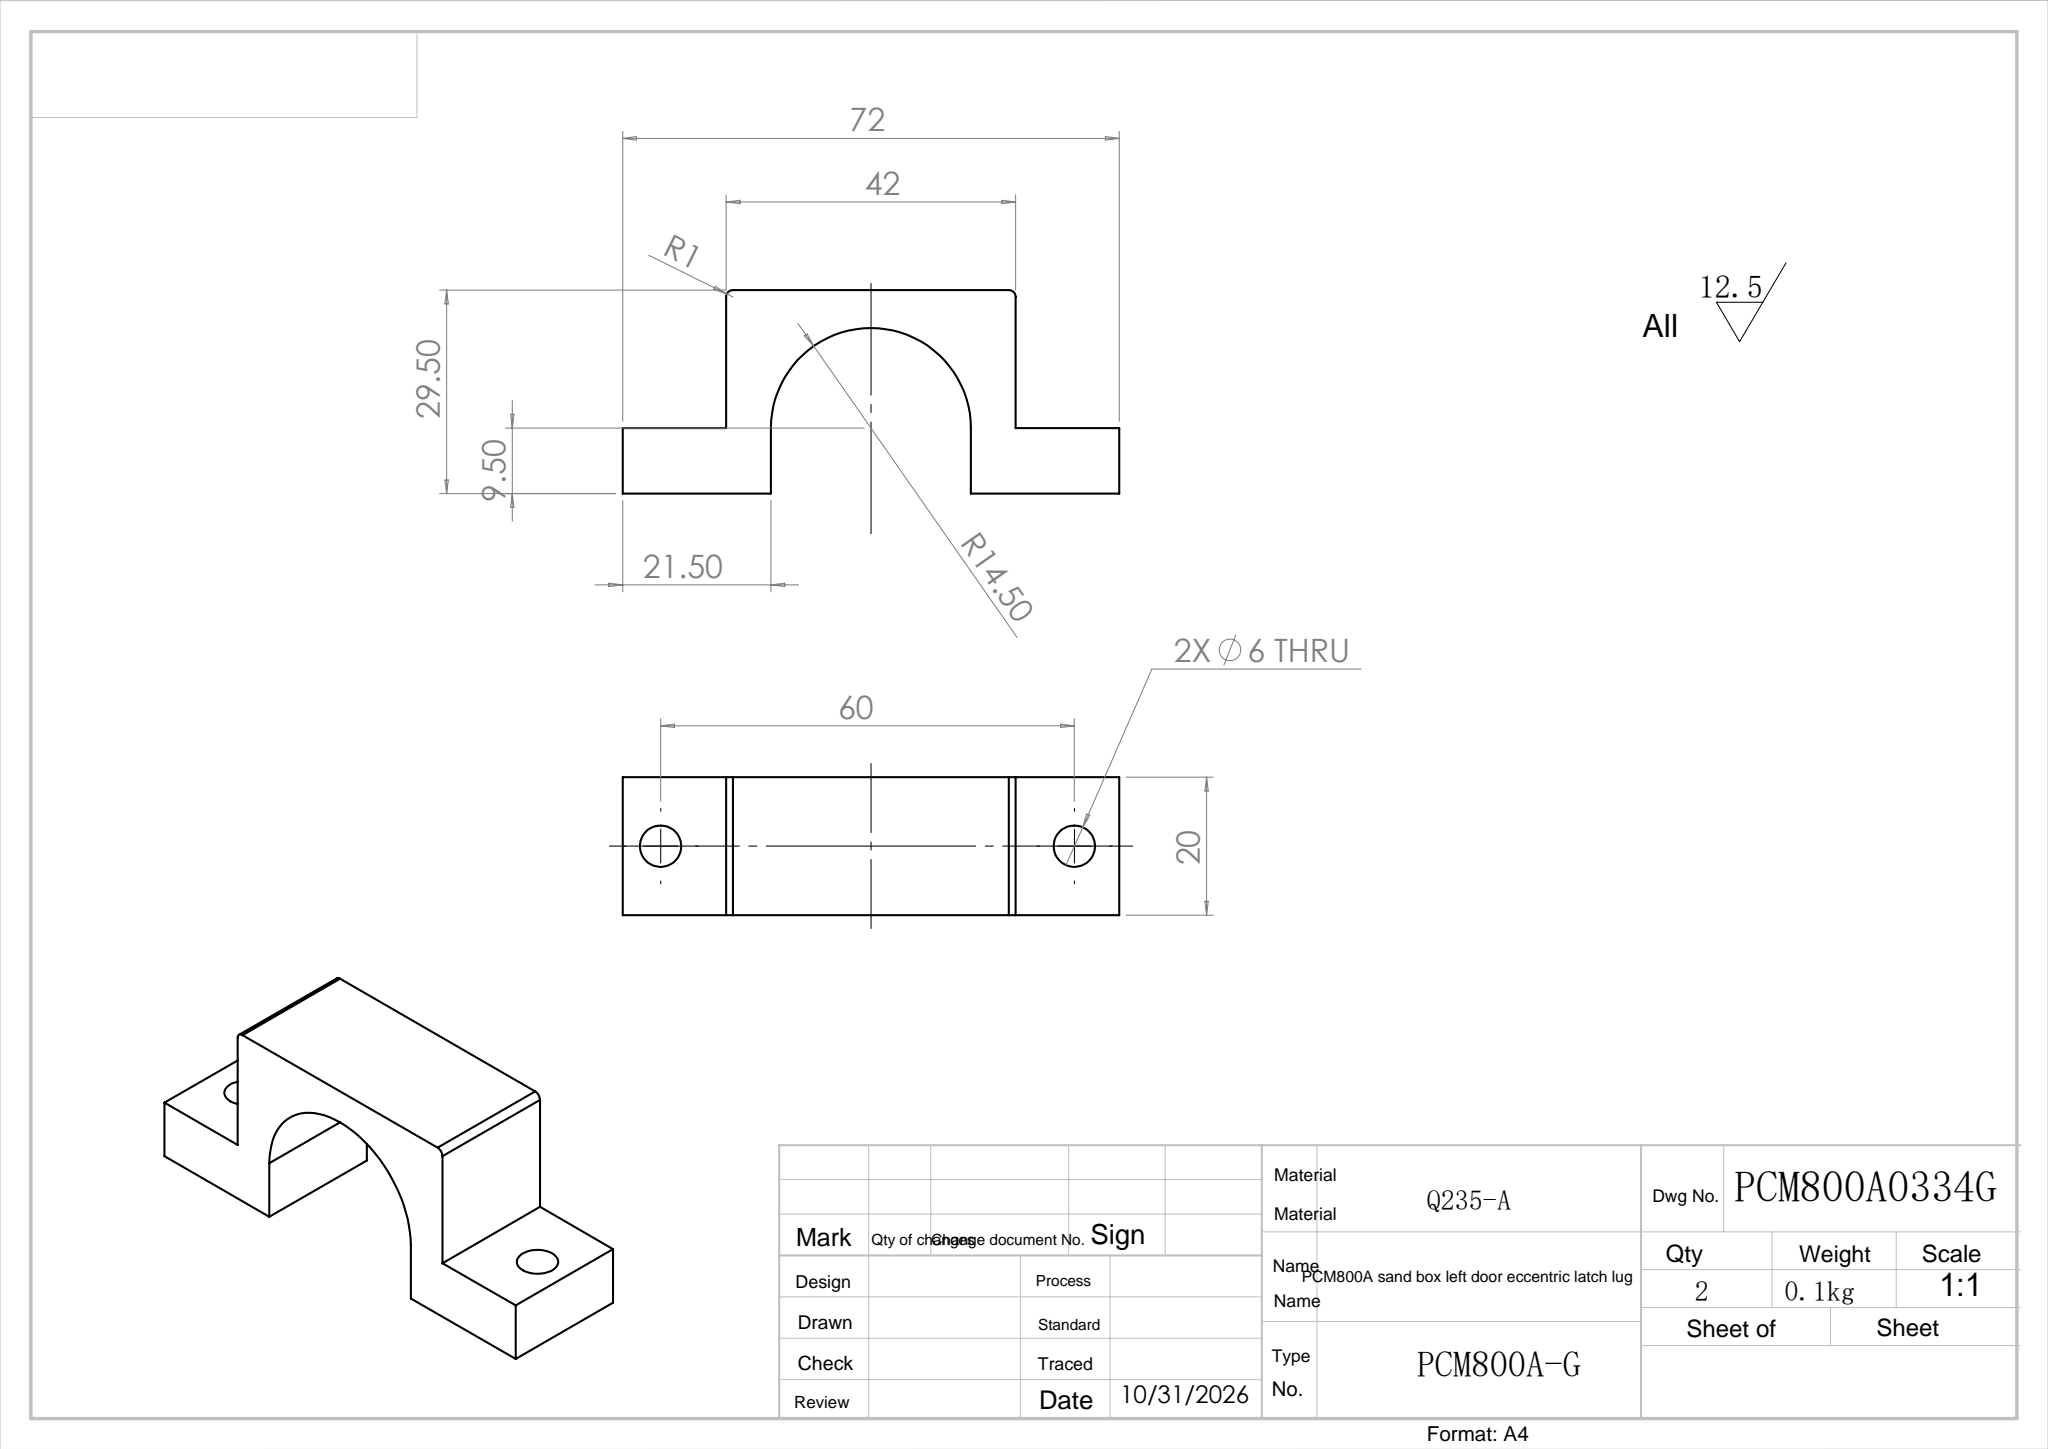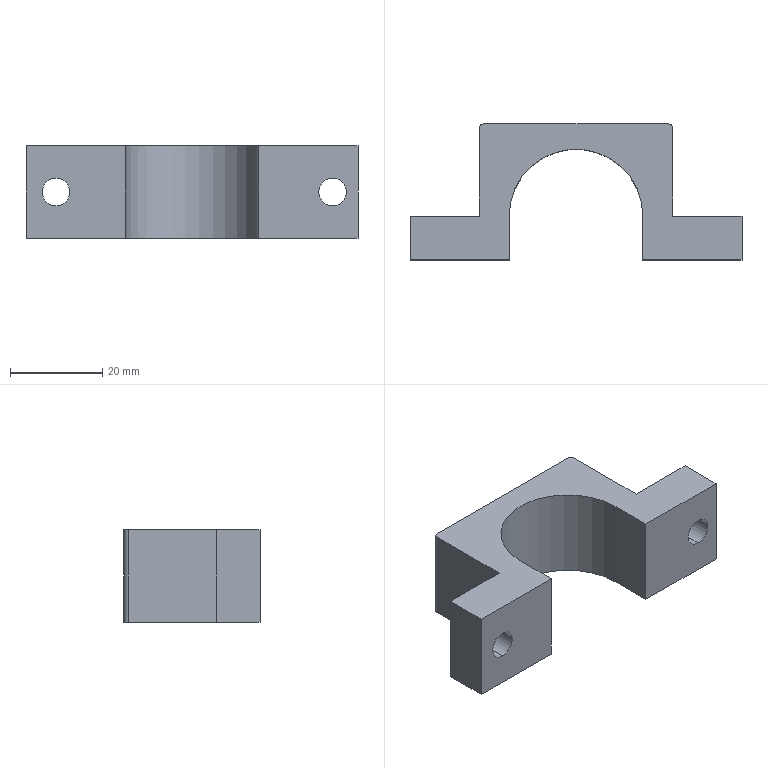Part | SolidWorks | features Extrusion 1, Fillet 1, ICE 1 | 1 solid | 20 faces | box 72 x 29.5 x 20 mm | volume 17819 mm3 | plane 13 | cylinder 7 | commonest cylinder face diameters 6 x4 2 x2 29 x1
STEP:
#1=CARTESIAN_POINT('',(66.5,-9.5,7.));
#2=VERTEX_POINT('',#1);
#3=CARTESIAN_POINT('',(66.5,-9.5,13.));
#4=VERTEX_POINT('',#3);
#5=CARTESIAN_POINT('',(66.5,-9.5,10.));
#6=DIRECTION('',(0.,1.,0.));
#7=DIRECTION('',(0.,0.,1.));
#8=AXIS2_PLACEMENT_3D('',#5,#6,#7);
#9=CIRCLE('',#8,3.);
#10=EDGE_CURVE('',#2,#4,#9,.T.);
#11=ORIENTED_EDGE('',*,*,#10,.F.);
#12=CARTESIAN_POINT('',(66.5,0.,7.));
#13=VERTEX_POINT('',#12);
#14=CARTESIAN_POINT('',(66.5,-9.5,7.));
#15=DIRECTION('',(0.,1.,0.));
#16=VECTOR('',#15,1000.);
#17=LINE('',#14,#16);
#18=EDGE_CURVE('',#2,#13,#17,.T.);
#19=ORIENTED_EDGE('',*,*,#18,.T.);
#20=CARTESIAN_POINT('',(66.5,0.,13.));
#21=VERTEX_POINT('',#20);
#22=CARTESIAN_POINT('',(66.5,0.,10.));
#23=DIRECTION('',(0.,1.,0.));
#24=DIRECTION('',(0.,0.,1.));
#25=AXIS2_PLACEMENT_3D('',#22,#23,#24);
#26=CIRCLE('',#25,3.);
#27=EDGE_CURVE('',#13,#21,#26,.T.);
#28=ORIENTED_EDGE('',*,*,#27,.T.);
#29=CARTESIAN_POINT('',(66.5,-9.5,13.));
#30=DIRECTION('',(0.,1.,0.));
#31=VECTOR('',#30,1000.);
#32=LINE('',#29,#31);
#33=EDGE_CURVE('',#4,#21,#32,.T.);
#34=ORIENTED_EDGE('',*,*,#33,.F.);
#35=EDGE_LOOP('',(#11,#19,#28,#34));
#36=FACE_OUTER_BOUND('',#35,.T.);
#37=CARTESIAN_POINT('',(66.5,-9.5,10.));
#38=DIRECTION('',(0.,1.,0.));
#39=DIRECTION('',(0.,0.,1.));
#40=AXIS2_PLACEMENT_3D('',#37,#38,#39);
#41=CYLINDRICAL_SURFACE('',#40,3.);
#42=ADVANCED_FACE('',(#36),#41,.F.);
#43=CARTESIAN_POINT('',(6.5,-9.5,7.));
#44=VERTEX_POINT('',#43);
#45=CARTESIAN_POINT('',(6.5,-9.5,13.));
#46=VERTEX_POINT('',#45);
#47=CARTESIAN_POINT('',(6.5,-9.5,10.));
#48=DIRECTION('',(0.,1.,0.));
#49=DIRECTION('',(0.,0.,1.));
#50=AXIS2_PLACEMENT_3D('',#47,#48,#49);
#51=CIRCLE('',#50,3.);
#52=EDGE_CURVE('',#44,#46,#51,.T.);
#53=ORIENTED_EDGE('',*,*,#52,.F.);
#54=CARTESIAN_POINT('',(6.5,0.,7.));
#55=VERTEX_POINT('',#54);
#56=CARTESIAN_POINT('',(6.5,-9.5,7.));
#57=DIRECTION('',(0.,1.,0.));
#58=VECTOR('',#57,1000.);
#59=LINE('',#56,#58);
#60=EDGE_CURVE('',#44,#55,#59,.T.);
#61=ORIENTED_EDGE('',*,*,#60,.T.);
#62=CARTESIAN_POINT('',(6.5,0.,13.));
#63=VERTEX_POINT('',#62);
#64=CARTESIAN_POINT('',(6.5,0.,10.));
#65=DIRECTION('',(0.,1.,0.));
#66=DIRECTION('',(0.,0.,1.));
#67=AXIS2_PLACEMENT_3D('',#64,#65,#66);
#68=CIRCLE('',#67,3.);
#69=EDGE_CURVE('',#55,#63,#68,.T.);
#70=ORIENTED_EDGE('',*,*,#69,.T.);
#71=CARTESIAN_POINT('',(6.5,-9.5,13.));
#72=DIRECTION('',(0.,1.,0.));
#73=VECTOR('',#72,1000.);
#74=LINE('',#71,#73);
#75=EDGE_CURVE('',#46,#63,#74,.T.);
#76=ORIENTED_EDGE('',*,*,#75,.F.);
#77=EDGE_LOOP('',(#53,#61,#70,#76));
#78=FACE_OUTER_BOUND('',#77,.T.);
#79=CARTESIAN_POINT('',(6.5,-9.5,10.));
#80=DIRECTION('',(0.,1.,0.));
#81=DIRECTION('',(0.,0.,1.));
#82=AXIS2_PLACEMENT_3D('',#79,#80,#81);
#83=CYLINDRICAL_SURFACE('',#82,3.);
#84=ADVANCED_FACE('',(#78),#83,.F.);
#85=CARTESIAN_POINT('',(0.,0.,0.));
#86=VERTEX_POINT('',#85);
#87=CARTESIAN_POINT('',(0.,-9.5,0.));
#88=VERTEX_POINT('',#87);
#89=CARTESIAN_POINT('',(0.,-9.5,0.));
#90=DIRECTION('',(0.,-1.,0.));
#91=VECTOR('',#90,1000.);
#92=LINE('',#89,#91);
#93=EDGE_CURVE('',#86,#88,#92,.T.);
#94=ORIENTED_EDGE('',*,*,#93,.T.);
#95=CARTESIAN_POINT('',(0.,-9.5,20.));
#96=VERTEX_POINT('',#95);
#97=CARTESIAN_POINT('',(0.,-9.5,20.));
#98=DIRECTION('',(0.,0.,-1.));
#99=VECTOR('',#98,1000.);
#100=LINE('',#97,#99);
#101=EDGE_CURVE('',#96,#88,#100,.T.);
#102=ORIENTED_EDGE('',*,*,#101,.F.);
#103=CARTESIAN_POINT('',(0.,0.,20.));
#104=VERTEX_POINT('',#103);
#105=CARTESIAN_POINT('',(0.,-9.5,20.));
#106=DIRECTION('',(0.,-1.,0.));
#107=VECTOR('',#106,1000.);
#108=LINE('',#105,#107);
#109=EDGE_CURVE('',#104,#96,#108,.T.);
#110=ORIENTED_EDGE('',*,*,#109,.F.);
#111=CARTESIAN_POINT('',(0.,0.,20.));
#112=DIRECTION('',(0.,0.,-1.));
#113=VECTOR('',#112,1000.);
#114=LINE('',#111,#113);
#115=EDGE_CURVE('',#104,#86,#114,.T.);
#116=ORIENTED_EDGE('',*,*,#115,.T.);
#117=EDGE_LOOP('',(#94,#102,#110,#116));
#118=FACE_OUTER_BOUND('',#117,.T.);
#119=CARTESIAN_POINT('',(0.,-9.5,20.));
#120=DIRECTION('',(1.,0.,0.));
#121=DIRECTION('',(0.,0.,-1.));
#122=AXIS2_PLACEMENT_3D('',#119,#120,#121);
#123=PLANE('',#122);
#124=ADVANCED_FACE('',(#118),#123,.F.);
#125=CARTESIAN_POINT('',(6.5,-9.5,10.));
#126=DIRECTION('',(0.,1.,0.));
#127=DIRECTION('',(0.,0.,1.));
#128=AXIS2_PLACEMENT_3D('',#125,#126,#127);
#129=CIRCLE('',#128,3.);
#130=EDGE_CURVE('',#46,#44,#129,.T.);
#131=ORIENTED_EDGE('',*,*,#130,.T.);
#132=ORIENTED_EDGE('',*,*,#52,.T.);
#133=EDGE_LOOP('',(#131,#132));
#134=FACE_BOUND('',#133,.T.);
#135=CARTESIAN_POINT('',(21.5,-9.5,0.));
#136=VERTEX_POINT('',#135);
#137=CARTESIAN_POINT('',(21.5,-9.5,0.));
#138=DIRECTION('',(1.,0.,0.));
#139=VECTOR('',#138,1000.);
#140=LINE('',#137,#139);
#141=EDGE_CURVE('',#88,#136,#140,.T.);
#142=ORIENTED_EDGE('',*,*,#141,.T.);
#143=CARTESIAN_POINT('',(21.5,-9.5,20.));
#144=VERTEX_POINT('',#143);
#145=CARTESIAN_POINT('',(21.5,-9.5,20.));
#146=DIRECTION('',(0.,0.,-1.));
#147=VECTOR('',#146,1000.);
#148=LINE('',#145,#147);
#149=EDGE_CURVE('',#144,#136,#148,.T.);
#150=ORIENTED_EDGE('',*,*,#149,.F.);
#151=CARTESIAN_POINT('',(21.5,-9.5,20.));
#152=DIRECTION('',(1.,0.,0.));
#153=VECTOR('',#152,1000.);
#154=LINE('',#151,#153);
#155=EDGE_CURVE('',#96,#144,#154,.T.);
#156=ORIENTED_EDGE('',*,*,#155,.F.);
#157=ORIENTED_EDGE('',*,*,#101,.T.);
#158=EDGE_LOOP('',(#142,#150,#156,#157));
#159=FACE_OUTER_BOUND('',#158,.T.);
#160=CARTESIAN_POINT('',(21.5,-9.5,20.));
#161=DIRECTION('',(0.,1.,0.));
#162=DIRECTION('',(-1.,0.,0.));
#163=AXIS2_PLACEMENT_3D('',#160,#161,#162);
#164=PLANE('',#163);
#165=ADVANCED_FACE('',(#134,#159),#164,.F.);
#166=CARTESIAN_POINT('',(21.5,0.,0.));
#167=VERTEX_POINT('',#166);
#168=CARTESIAN_POINT('',(21.5,0.,0.));
#169=DIRECTION('',(0.,1.,0.));
#170=VECTOR('',#169,1000.);
#171=LINE('',#168,#170);
#172=EDGE_CURVE('',#136,#167,#171,.T.);
#173=ORIENTED_EDGE('',*,*,#172,.T.);
#174=CARTESIAN_POINT('',(21.5,0.,20.));
#175=VERTEX_POINT('',#174);
#176=CARTESIAN_POINT('',(21.5,0.,20.));
#177=DIRECTION('',(0.,0.,-1.));
#178=VECTOR('',#177,1000.);
#179=LINE('',#176,#178);
#180=EDGE_CURVE('',#175,#167,#179,.T.);
#181=ORIENTED_EDGE('',*,*,#180,.F.);
#182=CARTESIAN_POINT('',(21.5,0.,20.));
#183=DIRECTION('',(0.,1.,0.));
#184=VECTOR('',#183,1000.);
#185=LINE('',#182,#184);
#186=EDGE_CURVE('',#144,#175,#185,.T.);
#187=ORIENTED_EDGE('',*,*,#186,.F.);
#188=ORIENTED_EDGE('',*,*,#149,.T.);
#189=EDGE_LOOP('',(#173,#181,#187,#188));
#190=FACE_OUTER_BOUND('',#189,.T.);
#191=CARTESIAN_POINT('',(21.5,0.,20.));
#192=DIRECTION('',(-1.,0.,0.));
#193=DIRECTION('',(0.,-1.,0.));
#194=AXIS2_PLACEMENT_3D('',#191,#192,#193);
#195=PLANE('',#194);
#196=ADVANCED_FACE('',(#190),#195,.F.);
#197=CARTESIAN_POINT('',(50.5,0.,0.));
#198=VERTEX_POINT('',#197);
#199=CARTESIAN_POINT('',(36.,0.,0.));
#200=DIRECTION('',(0.,0.,-1.));
#201=DIRECTION('',(1.,0.,0.));
#202=AXIS2_PLACEMENT_3D('',#199,#200,#201);
#203=CIRCLE('',#202,14.5);
#204=EDGE_CURVE('',#167,#198,#203,.T.);
#205=ORIENTED_EDGE('',*,*,#204,.T.);
#206=CARTESIAN_POINT('',(50.5,0.,20.));
#207=VERTEX_POINT('',#206);
#208=CARTESIAN_POINT('',(50.5,0.,20.));
#209=DIRECTION('',(0.,0.,-1.));
#210=VECTOR('',#209,1000.);
#211=LINE('',#208,#210);
#212=EDGE_CURVE('',#207,#198,#211,.T.);
#213=ORIENTED_EDGE('',*,*,#212,.F.);
#214=CARTESIAN_POINT('',(36.,0.,20.));
#215=DIRECTION('',(0.,0.,-1.));
#216=DIRECTION('',(1.,0.,0.));
#217=AXIS2_PLACEMENT_3D('',#214,#215,#216);
#218=CIRCLE('',#217,14.5);
#219=EDGE_CURVE('',#175,#207,#218,.T.);
#220=ORIENTED_EDGE('',*,*,#219,.F.);
#221=ORIENTED_EDGE('',*,*,#180,.T.);
#222=EDGE_LOOP('',(#205,#213,#220,#221));
#223=FACE_OUTER_BOUND('',#222,.T.);
#224=CARTESIAN_POINT('',(36.,0.,20.));
#225=DIRECTION('',(0.,0.,-1.));
#226=DIRECTION('',(-1.,0.,0.));
#227=AXIS2_PLACEMENT_3D('',#224,#225,#226);
#228=CYLINDRICAL_SURFACE('',#227,14.5);
#229=ADVANCED_FACE('',(#223),#228,.F.);
#230=CARTESIAN_POINT('',(50.5,-9.5,0.));
#231=VERTEX_POINT('',#230);
#232=CARTESIAN_POINT('',(50.5,0.,0.));
#233=DIRECTION('',(0.,-1.,0.));
#234=VECTOR('',#233,1000.);
#235=LINE('',#232,#234);
#236=EDGE_CURVE('',#198,#231,#235,.T.);
#237=ORIENTED_EDGE('',*,*,#236,.T.);
#238=CARTESIAN_POINT('',(50.5,-9.5,20.));
#239=VERTEX_POINT('',#238);
#240=CARTESIAN_POINT('',(50.5,-9.5,20.));
#241=DIRECTION('',(0.,0.,-1.));
#242=VECTOR('',#241,1000.);
#243=LINE('',#240,#242);
#244=EDGE_CURVE('',#239,#231,#243,.T.);
#245=ORIENTED_EDGE('',*,*,#244,.F.);
#246=CARTESIAN_POINT('',(50.5,0.,20.));
#247=DIRECTION('',(0.,-1.,0.));
#248=VECTOR('',#247,1000.);
#249=LINE('',#246,#248);
#250=EDGE_CURVE('',#207,#239,#249,.T.);
#251=ORIENTED_EDGE('',*,*,#250,.F.);
#252=ORIENTED_EDGE('',*,*,#212,.T.);
#253=EDGE_LOOP('',(#237,#245,#251,#252));
#254=FACE_OUTER_BOUND('',#253,.T.);
#255=CARTESIAN_POINT('',(50.5,0.,20.));
#256=DIRECTION('',(1.,0.,0.));
#257=DIRECTION('',(0.,1.,0.));
#258=AXIS2_PLACEMENT_3D('',#255,#256,#257);
#259=PLANE('',#258);
#260=ADVANCED_FACE('',(#254),#259,.F.);
#261=CARTESIAN_POINT('',(66.5,-9.5,10.));
#262=DIRECTION('',(0.,1.,0.));
#263=DIRECTION('',(0.,0.,1.));
#264=AXIS2_PLACEMENT_3D('',#261,#262,#263);
#265=CIRCLE('',#264,3.);
#266=EDGE_CURVE('',#4,#2,#265,.T.);
#267=ORIENTED_EDGE('',*,*,#266,.T.);
#268=ORIENTED_EDGE('',*,*,#10,.T.);
#269=EDGE_LOOP('',(#267,#268));
#270=FACE_BOUND('',#269,.T.);
#271=CARTESIAN_POINT('',(72.,-9.5,0.));
#272=VERTEX_POINT('',#271);
#273=CARTESIAN_POINT('',(72.,-9.5,0.));
#274=DIRECTION('',(1.,0.,0.));
#275=VECTOR('',#274,1000.);
#276=LINE('',#273,#275);
#277=EDGE_CURVE('',#231,#272,#276,.T.);
#278=ORIENTED_EDGE('',*,*,#277,.T.);
#279=CARTESIAN_POINT('',(72.,-9.5,20.));
#280=VERTEX_POINT('',#279);
#281=CARTESIAN_POINT('',(72.,-9.5,20.));
#282=DIRECTION('',(0.,0.,-1.));
#283=VECTOR('',#282,1000.);
#284=LINE('',#281,#283);
#285=EDGE_CURVE('',#280,#272,#284,.T.);
#286=ORIENTED_EDGE('',*,*,#285,.F.);
#287=CARTESIAN_POINT('',(72.,-9.5,20.));
#288=DIRECTION('',(1.,0.,0.));
#289=VECTOR('',#288,1000.);
#290=LINE('',#287,#289);
#291=EDGE_CURVE('',#239,#280,#290,.T.);
#292=ORIENTED_EDGE('',*,*,#291,.F.);
#293=ORIENTED_EDGE('',*,*,#244,.T.);
#294=EDGE_LOOP('',(#278,#286,#292,#293));
#295=FACE_OUTER_BOUND('',#294,.T.);
#296=CARTESIAN_POINT('',(72.,-9.5,20.));
#297=DIRECTION('',(0.,1.,0.));
#298=DIRECTION('',(0.,0.,1.));
#299=AXIS2_PLACEMENT_3D('',#296,#297,#298);
#300=PLANE('',#299);
#301=ADVANCED_FACE('',(#270,#295),#300,.F.);
#302=CARTESIAN_POINT('',(72.,0.,0.));
#303=VERTEX_POINT('',#302);
#304=CARTESIAN_POINT('',(72.,0.,0.));
#305=DIRECTION('',(0.,1.,0.));
#306=VECTOR('',#305,1000.);
#307=LINE('',#304,#306);
#308=EDGE_CURVE('',#272,#303,#307,.T.);
#309=ORIENTED_EDGE('',*,*,#308,.T.);
#310=CARTESIAN_POINT('',(72.,0.,20.));
#311=VERTEX_POINT('',#310);
#312=CARTESIAN_POINT('',(72.,0.,20.));
#313=DIRECTION('',(0.,0.,-1.));
#314=VECTOR('',#313,1000.);
#315=LINE('',#312,#314);
#316=EDGE_CURVE('',#311,#303,#315,.T.);
#317=ORIENTED_EDGE('',*,*,#316,.F.);
#318=CARTESIAN_POINT('',(72.,0.,20.));
#319=DIRECTION('',(0.,1.,0.));
#320=VECTOR('',#319,1000.);
#321=LINE('',#318,#320);
#322=EDGE_CURVE('',#280,#311,#321,.T.);
#323=ORIENTED_EDGE('',*,*,#322,.F.);
#324=ORIENTED_EDGE('',*,*,#285,.T.);
#325=EDGE_LOOP('',(#309,#317,#323,#324));
#326=FACE_OUTER_BOUND('',#325,.T.);
#327=CARTESIAN_POINT('',(72.,0.,20.));
#328=DIRECTION('',(-1.,0.,0.));
#329=DIRECTION('',(0.,0.,1.));
#330=AXIS2_PLACEMENT_3D('',#327,#328,#329);
#331=PLANE('',#330);
#332=ADVANCED_FACE('',(#326),#331,.F.);
#333=CARTESIAN_POINT('',(66.5,0.,10.));
#334=DIRECTION('',(0.,1.,0.));
#335=DIRECTION('',(0.,0.,1.));
#336=AXIS2_PLACEMENT_3D('',#333,#334,#335);
#337=CIRCLE('',#336,3.);
#338=EDGE_CURVE('',#21,#13,#337,.T.);
#339=ORIENTED_EDGE('',*,*,#338,.F.);
#340=ORIENTED_EDGE('',*,*,#27,.F.);
#341=EDGE_LOOP('',(#339,#340));
#342=FACE_BOUND('',#341,.T.);
#343=CARTESIAN_POINT('',(57.,0.,0.));
#344=VERTEX_POINT('',#343);
#345=CARTESIAN_POINT('',(57.,0.,0.));
#346=DIRECTION('',(-1.,0.,0.));
#347=VECTOR('',#346,1000.);
#348=LINE('',#345,#347);
#349=EDGE_CURVE('',#303,#344,#348,.T.);
#350=ORIENTED_EDGE('',*,*,#349,.T.);
#351=CARTESIAN_POINT('',(57.,0.,20.));
#352=VERTEX_POINT('',#351);
#353=CARTESIAN_POINT('',(57.,0.,20.));
#354=DIRECTION('',(0.,0.,-1.));
#355=VECTOR('',#354,1000.);
#356=LINE('',#353,#355);
#357=EDGE_CURVE('',#352,#344,#356,.T.);
#358=ORIENTED_EDGE('',*,*,#357,.F.);
#359=CARTESIAN_POINT('',(57.,0.,20.));
#360=DIRECTION('',(-1.,0.,0.));
#361=VECTOR('',#360,1000.);
#362=LINE('',#359,#361);
#363=EDGE_CURVE('',#311,#352,#362,.T.);
#364=ORIENTED_EDGE('',*,*,#363,.F.);
#365=ORIENTED_EDGE('',*,*,#316,.T.);
#366=EDGE_LOOP('',(#350,#358,#364,#365));
#367=FACE_OUTER_BOUND('',#366,.T.);
#368=CARTESIAN_POINT('',(57.,0.,20.));
#369=DIRECTION('',(0.,-1.,0.));
#370=DIRECTION('',(0.,0.,-1.));
#371=AXIS2_PLACEMENT_3D('',#368,#369,#370);
#372=PLANE('',#371);
#373=ADVANCED_FACE('',(#342,#367),#372,.F.);
#374=CARTESIAN_POINT('',(57.,19.,0.));
#375=VERTEX_POINT('',#374);
#376=CARTESIAN_POINT('',(57.,20.,0.));
#377=DIRECTION('',(0.,1.,0.));
#378=VECTOR('',#377,1000.);
#379=LINE('',#376,#378);
#380=EDGE_CURVE('',#344,#375,#379,.T.);
#381=ORIENTED_EDGE('',*,*,#380,.T.);
#382=CARTESIAN_POINT('',(57.,19.,20.));
#383=VERTEX_POINT('',#382);
#384=CARTESIAN_POINT('',(57.,19.,20.));
#385=DIRECTION('',(0.,0.,1.));
#386=VECTOR('',#385,1000.);
#387=LINE('',#384,#386);
#388=EDGE_CURVE('',#375,#383,#387,.T.);
#389=ORIENTED_EDGE('',*,*,#388,.T.);
#390=CARTESIAN_POINT('',(57.,20.,20.));
#391=DIRECTION('',(0.,1.,0.));
#392=VECTOR('',#391,1000.);
#393=LINE('',#390,#392);
#394=EDGE_CURVE('',#352,#383,#393,.T.);
#395=ORIENTED_EDGE('',*,*,#394,.F.);
#396=ORIENTED_EDGE('',*,*,#357,.T.);
#397=EDGE_LOOP('',(#381,#389,#395,#396));
#398=FACE_OUTER_BOUND('',#397,.T.);
#399=CARTESIAN_POINT('',(57.,20.,20.));
#400=DIRECTION('',(-1.,0.,0.));
#401=DIRECTION('',(0.,-1.,0.));
#402=AXIS2_PLACEMENT_3D('',#399,#400,#401);
#403=PLANE('',#402);
#404=ADVANCED_FACE('',(#398),#403,.F.);
#405=CARTESIAN_POINT('',(56.,20.,20.));
#406=VERTEX_POINT('',#405);
#407=CARTESIAN_POINT('',(16.,20.,20.));
#408=VERTEX_POINT('',#407);
#409=CARTESIAN_POINT('',(15.,20.,20.));
#410=DIRECTION('',(-1.,0.,0.));
#411=VECTOR('',#410,1000.);
#412=LINE('',#409,#411);
#413=EDGE_CURVE('',#406,#408,#412,.T.);
#414=ORIENTED_EDGE('',*,*,#413,.F.);
#415=CARTESIAN_POINT('',(56.,20.,0.));
#416=VERTEX_POINT('',#415);
#417=CARTESIAN_POINT('',(56.,20.,20.));
#418=DIRECTION('',(0.,0.,-1.));
#419=VECTOR('',#418,1000.);
#420=LINE('',#417,#419);
#421=EDGE_CURVE('',#406,#416,#420,.T.);
#422=ORIENTED_EDGE('',*,*,#421,.T.);
#423=CARTESIAN_POINT('',(16.,20.,0.));
#424=VERTEX_POINT('',#423);
#425=CARTESIAN_POINT('',(15.,20.,0.));
#426=DIRECTION('',(-1.,0.,0.));
#427=VECTOR('',#426,1000.);
#428=LINE('',#425,#427);
#429=EDGE_CURVE('',#416,#424,#428,.T.);
#430=ORIENTED_EDGE('',*,*,#429,.T.);
#431=CARTESIAN_POINT('',(16.,20.,20.));
#432=DIRECTION('',(0.,0.,1.));
#433=VECTOR('',#432,1000.);
#434=LINE('',#431,#433);
#435=EDGE_CURVE('',#424,#408,#434,.T.);
#436=ORIENTED_EDGE('',*,*,#435,.T.);
#437=EDGE_LOOP('',(#414,#422,#430,#436));
#438=FACE_OUTER_BOUND('',#437,.T.);
#439=CARTESIAN_POINT('',(15.,20.,20.));
#440=DIRECTION('',(0.,-1.,0.));
#441=DIRECTION('',(0.,0.,-1.));
#442=AXIS2_PLACEMENT_3D('',#439,#440,#441);
#443=PLANE('',#442);
#444=ADVANCED_FACE('',(#438),#443,.F.);
#445=CARTESIAN_POINT('',(15.,19.,20.));
#446=VERTEX_POINT('',#445);
#447=CARTESIAN_POINT('',(15.,0.,20.));
#448=VERTEX_POINT('',#447);
#449=CARTESIAN_POINT('',(15.,0.,20.));
#450=DIRECTION('',(0.,-1.,0.));
#451=VECTOR('',#450,1000.);
#452=LINE('',#449,#451);
#453=EDGE_CURVE('',#446,#448,#452,.T.);
#454=ORIENTED_EDGE('',*,*,#453,.F.);
#455=CARTESIAN_POINT('',(15.,19.,0.));
#456=VERTEX_POINT('',#455);
#457=CARTESIAN_POINT('',(15.,19.,20.));
#458=DIRECTION('',(0.,0.,-1.));
#459=VECTOR('',#458,1000.);
#460=LINE('',#457,#459);
#461=EDGE_CURVE('',#446,#456,#460,.T.);
#462=ORIENTED_EDGE('',*,*,#461,.T.);
#463=CARTESIAN_POINT('',(15.,0.,0.));
#464=VERTEX_POINT('',#463);
#465=CARTESIAN_POINT('',(15.,0.,0.));
#466=DIRECTION('',(0.,-1.,0.));
#467=VECTOR('',#466,1000.);
#468=LINE('',#465,#467);
#469=EDGE_CURVE('',#456,#464,#468,.T.);
#470=ORIENTED_EDGE('',*,*,#469,.T.);
#471=CARTESIAN_POINT('',(15.,0.,20.));
#472=DIRECTION('',(0.,0.,-1.));
#473=VECTOR('',#472,1000.);
#474=LINE('',#471,#473);
#475=EDGE_CURVE('',#448,#464,#474,.T.);
#476=ORIENTED_EDGE('',*,*,#475,.F.);
#477=EDGE_LOOP('',(#454,#462,#470,#476));
#478=FACE_OUTER_BOUND('',#477,.T.);
#479=CARTESIAN_POINT('',(15.,0.,20.));
#480=DIRECTION('',(1.,0.,0.));
#481=DIRECTION('',(0.,0.,-1.));
#482=AXIS2_PLACEMENT_3D('',#479,#480,#481);
#483=PLANE('',#482);
#484=ADVANCED_FACE('',(#478),#483,.F.);
#485=CARTESIAN_POINT('',(6.5,0.,10.));
#486=DIRECTION('',(0.,1.,0.));
#487=DIRECTION('',(0.,0.,1.));
#488=AXIS2_PLACEMENT_3D('',#485,#486,#487);
#489=CIRCLE('',#488,3.);
#490=EDGE_CURVE('',#63,#55,#489,.T.);
#491=ORIENTED_EDGE('',*,*,#490,.F.);
#492=ORIENTED_EDGE('',*,*,#69,.F.);
#493=EDGE_LOOP('',(#491,#492));
#494=FACE_BOUND('',#493,.T.);
#495=CARTESIAN_POINT('',(0.,0.,0.));
#496=DIRECTION('',(-1.,0.,0.));
#497=VECTOR('',#496,1000.);
#498=LINE('',#495,#497);
#499=EDGE_CURVE('',#464,#86,#498,.T.);
#500=ORIENTED_EDGE('',*,*,#499,.T.);
#501=ORIENTED_EDGE('',*,*,#115,.F.);
#502=CARTESIAN_POINT('',(0.,0.,20.));
#503=DIRECTION('',(-1.,0.,0.));
#504=VECTOR('',#503,1000.);
#505=LINE('',#502,#504);
#506=EDGE_CURVE('',#448,#104,#505,.T.);
#507=ORIENTED_EDGE('',*,*,#506,.F.);
#508=ORIENTED_EDGE('',*,*,#475,.T.);
#509=EDGE_LOOP('',(#500,#501,#507,#508));
#510=FACE_OUTER_BOUND('',#509,.T.);
#511=CARTESIAN_POINT('',(0.,0.,20.));
#512=DIRECTION('',(0.,-1.,0.));
#513=DIRECTION('',(0.,0.,-1.));
#514=AXIS2_PLACEMENT_3D('',#511,#512,#513);
#515=PLANE('',#514);
#516=ADVANCED_FACE('',(#494,#510),#515,.F.);
#517=ORIENTED_EDGE('',*,*,#394,.T.);
#518=CARTESIAN_POINT('',(56.,19.,20.));
#519=DIRECTION('',(0.,0.,1.));
#520=DIRECTION('',(1.,0.,0.));
#521=AXIS2_PLACEMENT_3D('',#518,#519,#520);
#522=CIRCLE('',#521,1.);
#523=EDGE_CURVE('',#383,#406,#522,.T.);
#524=ORIENTED_EDGE('',*,*,#523,.T.);
#525=ORIENTED_EDGE('',*,*,#413,.T.);
#526=CARTESIAN_POINT('',(16.,19.,20.));
#527=DIRECTION('',(0.,0.,1.));
#528=DIRECTION('',(1.,0.,0.));
#529=AXIS2_PLACEMENT_3D('',#526,#527,#528);
#530=CIRCLE('',#529,1.);
#531=EDGE_CURVE('',#408,#446,#530,.T.);
#532=ORIENTED_EDGE('',*,*,#531,.T.);
#533=ORIENTED_EDGE('',*,*,#453,.T.);
#534=ORIENTED_EDGE('',*,*,#506,.T.);
#535=ORIENTED_EDGE('',*,*,#109,.T.);
#536=ORIENTED_EDGE('',*,*,#155,.T.);
#537=ORIENTED_EDGE('',*,*,#186,.T.);
#538=ORIENTED_EDGE('',*,*,#219,.T.);
#539=ORIENTED_EDGE('',*,*,#250,.T.);
#540=ORIENTED_EDGE('',*,*,#291,.T.);
#541=ORIENTED_EDGE('',*,*,#322,.T.);
#542=ORIENTED_EDGE('',*,*,#363,.T.);
#543=EDGE_LOOP('',(#517,#524,#525,#532,#533,#534,#535,#536,#537,#538,#539,#540,#541,#542));
#544=FACE_OUTER_BOUND('',#543,.T.);
#545=CARTESIAN_POINT('',(36.,0.,20.));
#546=DIRECTION('',(0.,0.,1.));
#547=DIRECTION('',(1.,0.,0.));
#548=AXIS2_PLACEMENT_3D('',#545,#546,#547);
#549=PLANE('',#548);
#550=ADVANCED_FACE('',(#544),#549,.T.);
#551=ORIENTED_EDGE('',*,*,#429,.F.);
#552=CARTESIAN_POINT('',(56.,19.,0.));
#553=DIRECTION('',(0.,0.,-1.));
#554=DIRECTION('',(1.,0.,0.));
#555=AXIS2_PLACEMENT_3D('',#552,#553,#554);
#556=CIRCLE('',#555,1.);
#557=EDGE_CURVE('',#416,#375,#556,.T.);
#558=ORIENTED_EDGE('',*,*,#557,.T.);
#559=ORIENTED_EDGE('',*,*,#380,.F.);
#560=ORIENTED_EDGE('',*,*,#349,.F.);
#561=ORIENTED_EDGE('',*,*,#308,.F.);
#562=ORIENTED_EDGE('',*,*,#277,.F.);
#563=ORIENTED_EDGE('',*,*,#236,.F.);
#564=ORIENTED_EDGE('',*,*,#204,.F.);
#565=ORIENTED_EDGE('',*,*,#172,.F.);
#566=ORIENTED_EDGE('',*,*,#141,.F.);
#567=ORIENTED_EDGE('',*,*,#93,.F.);
#568=ORIENTED_EDGE('',*,*,#499,.F.);
#569=ORIENTED_EDGE('',*,*,#469,.F.);
#570=CARTESIAN_POINT('',(16.,19.,0.));
#571=DIRECTION('',(0.,0.,-1.));
#572=DIRECTION('',(1.,0.,0.));
#573=AXIS2_PLACEMENT_3D('',#570,#571,#572);
#574=CIRCLE('',#573,1.);
#575=EDGE_CURVE('',#456,#424,#574,.T.);
#576=ORIENTED_EDGE('',*,*,#575,.T.);
#577=EDGE_LOOP('',(#551,#558,#559,#560,#561,#562,#563,#564,#565,#566,#567,#568,#569,#576));
#578=FACE_OUTER_BOUND('',#577,.T.);
#579=CARTESIAN_POINT('',(36.,0.,0.));
#580=DIRECTION('',(0.,0.,1.));
#581=DIRECTION('',(1.,0.,0.));
#582=AXIS2_PLACEMENT_3D('',#579,#580,#581);
#583=PLANE('',#582);
#584=ADVANCED_FACE('',(#578),#583,.F.);
#585=ORIENTED_EDGE('',*,*,#523,.F.);
#586=ORIENTED_EDGE('',*,*,#388,.F.);
#587=ORIENTED_EDGE('',*,*,#557,.F.);
#588=ORIENTED_EDGE('',*,*,#421,.F.);
#589=EDGE_LOOP('',(#585,#586,#587,#588));
#590=FACE_OUTER_BOUND('',#589,.T.);
#591=CARTESIAN_POINT('',(56.,19.,20.));
#592=DIRECTION('',(0.,0.,-1.));
#593=DIRECTION('',(-1.,0.,0.));
#594=AXIS2_PLACEMENT_3D('',#591,#592,#593);
#595=CYLINDRICAL_SURFACE('',#594,1.);
#596=ADVANCED_FACE('',(#590),#595,.T.);
#597=ORIENTED_EDGE('',*,*,#531,.F.);
#598=ORIENTED_EDGE('',*,*,#435,.F.);
#599=ORIENTED_EDGE('',*,*,#575,.F.);
#600=ORIENTED_EDGE('',*,*,#461,.F.);
#601=EDGE_LOOP('',(#597,#598,#599,#600));
#602=FACE_OUTER_BOUND('',#601,.T.);
#603=CARTESIAN_POINT('',(16.,19.,20.));
#604=DIRECTION('',(0.,0.,-1.));
#605=DIRECTION('',(-1.,0.,0.));
#606=AXIS2_PLACEMENT_3D('',#603,#604,#605);
#607=CYLINDRICAL_SURFACE('',#606,1.);
#608=ADVANCED_FACE('',(#602),#607,.T.);
#609=ORIENTED_EDGE('',*,*,#60,.F.);
#610=ORIENTED_EDGE('',*,*,#130,.F.);
#611=ORIENTED_EDGE('',*,*,#75,.T.);
#612=ORIENTED_EDGE('',*,*,#490,.T.);
#613=EDGE_LOOP('',(#609,#610,#611,#612));
#614=FACE_OUTER_BOUND('',#613,.T.);
#615=CARTESIAN_POINT('',(6.5,-9.5,10.));
#616=DIRECTION('',(0.,1.,0.));
#617=DIRECTION('',(0.,0.,1.));
#618=AXIS2_PLACEMENT_3D('',#615,#616,#617);
#619=CYLINDRICAL_SURFACE('',#618,3.);
#620=ADVANCED_FACE('',(#614),#619,.F.);
#621=ORIENTED_EDGE('',*,*,#18,.F.);
#622=ORIENTED_EDGE('',*,*,#266,.F.);
#623=ORIENTED_EDGE('',*,*,#33,.T.);
#624=ORIENTED_EDGE('',*,*,#338,.T.);
#625=EDGE_LOOP('',(#621,#622,#623,#624));
#626=FACE_OUTER_BOUND('',#625,.T.);
#627=CARTESIAN_POINT('',(66.5,-9.5,10.));
#628=DIRECTION('',(0.,1.,0.));
#629=DIRECTION('',(0.,0.,1.));
#630=AXIS2_PLACEMENT_3D('',#627,#628,#629);
#631=CYLINDRICAL_SURFACE('',#630,3.);
#632=ADVANCED_FACE('',(#626),#631,.F.);
#633=CLOSED_SHELL('',(#42,#84,#124,#165,#196,#229,#260,#301,#332,#373,#404,#444,#484,#516,#550,#584,#596,#608,#620,#632));
#634=MANIFOLD_SOLID_BREP('',#633);
#635=CARTESIAN_POINT('',(0.,0.,0.));
#636=DIRECTION('',(0.,0.,1.));
#637=DIRECTION('',(1.,0.,0.));
#638=AXIS2_PLACEMENT_3D('',#635,#636,#637);
#639=(LENGTH_UNIT()NAMED_UNIT(*)SI_UNIT(.MILLI.,.METRE.));
#640=UNCERTAINTY_MEASURE_WITH_UNIT(LENGTH_MEASURE(0.00001),#639,'','');
#641=(NAMED_UNIT(*)PLANE_ANGLE_UNIT()SI_UNIT($,.RADIAN.));
#642=(NAMED_UNIT(*)SI_UNIT($,.STERADIAN.)SOLID_ANGLE_UNIT());
#643=(GEOMETRIC_REPRESENTATION_CONTEXT(3)GLOBAL_UNCERTAINTY_ASSIGNED_CONTEXT((#640))GLOBAL_UNIT_ASSIGNED_CONTEXT((#639,#641,#642))REPRESENTATION_CONTEXT('',''));
#644=ADVANCED_BREP_SHAPE_REPRESENTATION('',(#634,#638),#643);